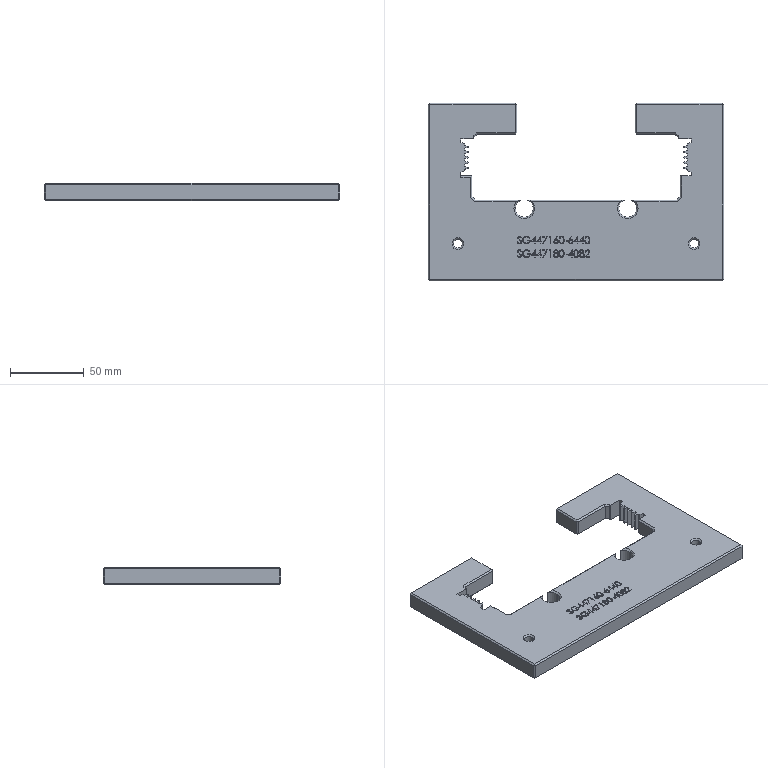Part | STEP file | Rotor mismatch gauge 3 | 1 solid | 500 faces | box 200 x 120 x 12 mm | volume 185482 mm3 | plane 328 | spline 142 | cone 20 | cylinder 10 | commonest cylinder face diameters 12 x6 6 x4